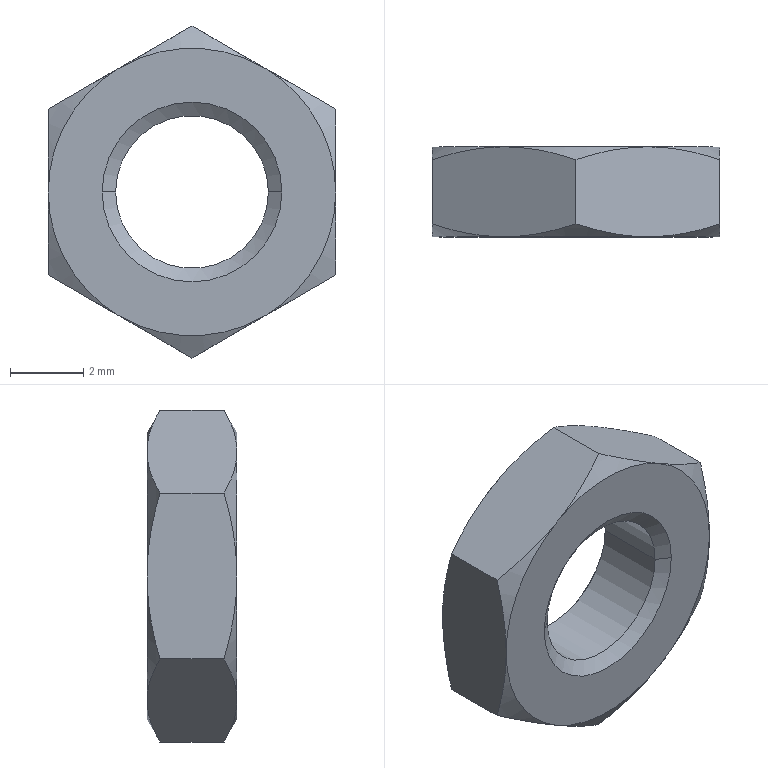Part | STEP file | 1 solid | 28 faces | box 7.84 x 2.45 x 9.053 mm | volume 94.615 mm3 | cone 16 | plane 8 | cylinder 4 | commonest cylinder face diameters 4.165 x2 4.9 x2